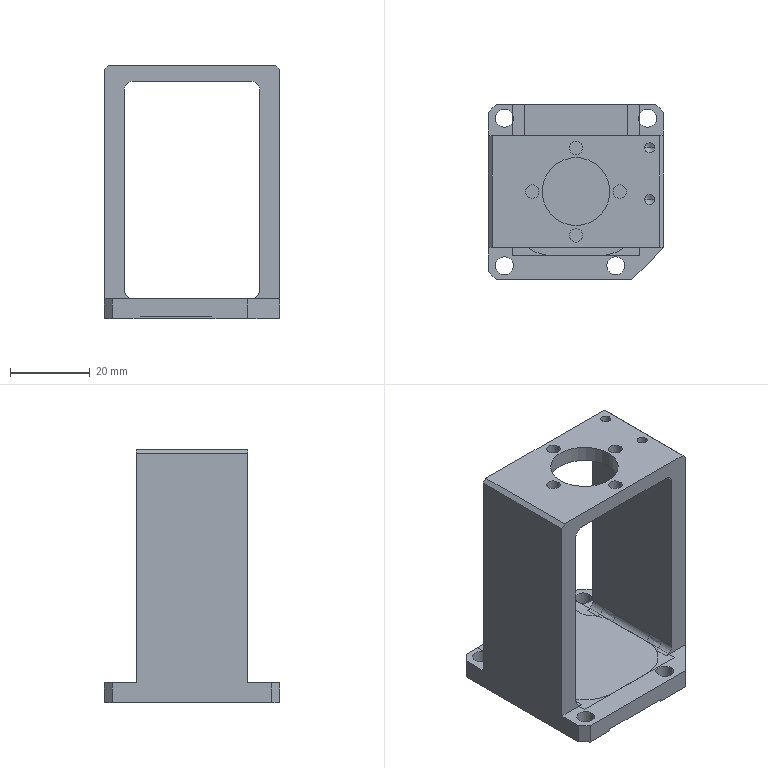NC program | NX | posted with a generic post | part box 44 x 44 x 63.6 mm
Lines 4428 to 4449 of 4449:
(PLANAR_MILL_COPY_1_1_COPY_1 , TOOL : D6A45)
N8848 T07 M6
N8850 G54
N8852 G17 G0 G90 X-22.1 Y-14.83 B0. C0. S9500 M3
N8854 G43 Z30. H7
N8856 Z-7.5
N8858 G94 G1 Z-9. F1250.
N8860 X-22.8 Y-15.234
N8862 G3 X-23.3 Y-16.1 R1.
N8864 G1 X25.8
N8866 G3 X26.9 Y-15. R1.1
N8868 G1 Y15.
N8870 G3 X25.8 Y16.1 R1.1
N8872 G1 X-23.3
N8874 G3 X-22.8 Y15.234 R1.
N8876 G1 X-22.1 Y14.83
N8878 Z-7.5
N8880 G0 Z30.
N8882 M5
N8884 M2